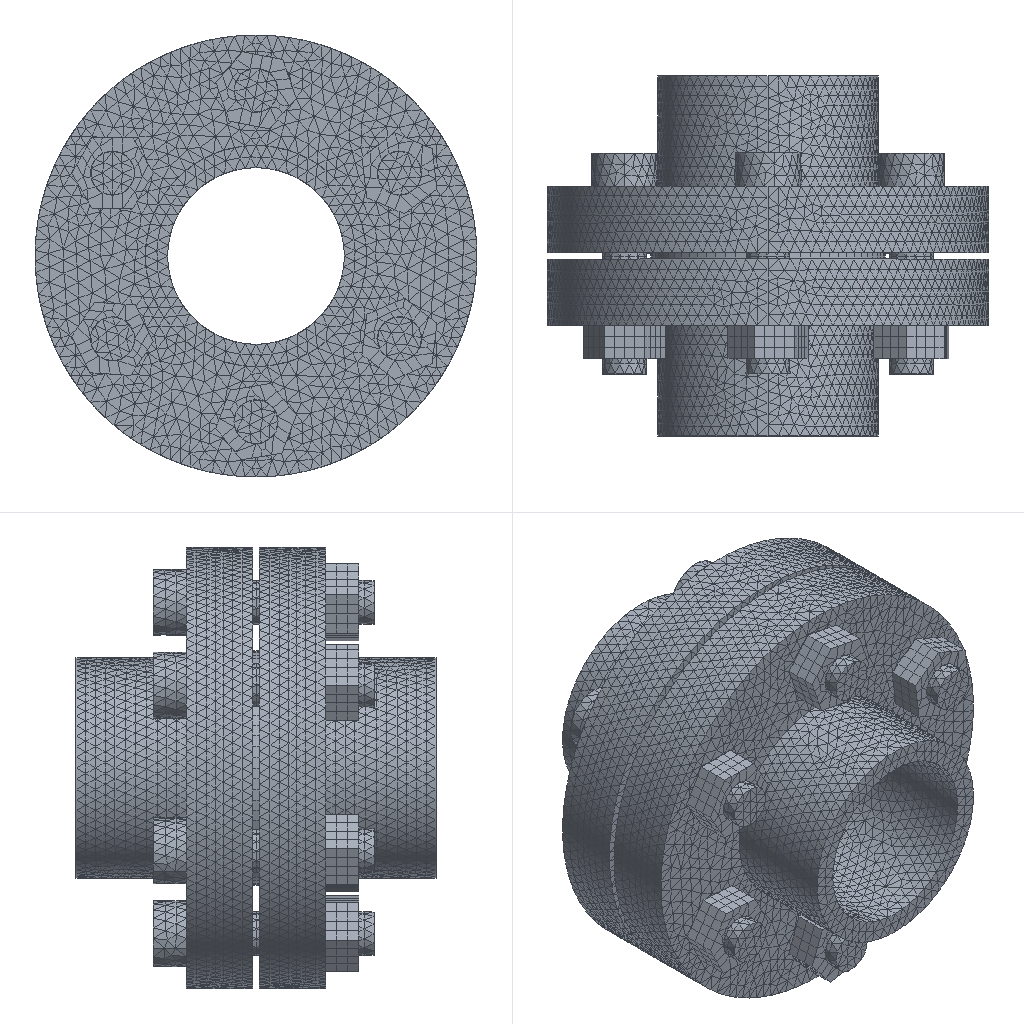Simulation study | ansys workbench
Set-up summary:
category,name,step,type,value,unit,region
solver,ansys_workbench
units,mm-N-s-tonne (MPa),,stated,"/units,MPA"
analysis,LS1,,static
load_step,LS1,LS1,static,nsubst=1; time=1
load_step,LS2,LS2,static,nsubst=1; time=2
mesh,nodes,,,141271
mesh,elements,,,93836
element_type,SOLID187,,,84073
element_type,SURF154,,,4096
element_type,TARGE170,,,2487
element_type,CONTA174,,,2487
element_type,SOLID186,,,693
material,Structural Steel,,E,200000,tonne s^-2 mm^-1
material,Structural Steel,,nu,0.3
material,Structural Steel,,density,7.85e-09,tonne mm^-3
material,Structural Steel,,conductivity,60.5,tonne mm s^-3 C^-1
material,Structural Steel,,specific_heat,4.34e+08,mm^2 s^-2 C^-1
material,Structural Steel,,cte,1.2e-05,C^-1
material,Structural Steel,,permeability,10000
material,Structural Steel,,resistivity,0.00017,ohm mm
material,Y?,,E,43,tonne s^-2 mm^-1
material,Y?,,nu,0.4995
material,Y?,,density,1.2e-09,tonne mm^-3
load,Define Pressure Using Surface Effect Elements,LS1,pressure,0.6,,SURF154 #44
load,Define Force Using Surface Effect Elements,LS1,surface-effect pres face 2,-18.392,,SURF154 #45
load,Define Force Using Surface Effect Elements,LS1,surface-effect pres face 2,-26.88,,SURF154 #46
load,Define Force Using Surface Effect Elements,LS1,surface-effect pres face 2,-26.88,,SURF154 #47
load,Define Force Using Surface Effect Elements,LS1,surface-effect pres face 2,-35.368,,SURF154 #48
load,Define Force Using Surface Effect Elements,LS1,surface-effect pres face 2,-26.88,,SURF154 #49
load,Define Force Using Surface Effect Elements,LS1,surface-effect pres face 2,-26.88,,SURF154 #50
bc,Fixed Supports,model,fixed,[dofs=ALL],,_FIXEDSU
contact,Contact Region,,bonded (always),element=CONTA174
contact,Contact Region 2,,bonded (always),element=CONTA174
contact,Contact Region 3,,bonded (always),element=CONTA174
contact,Contact Region 4,,bonded (always),element=CONTA174
contact,Contact Region 5,,bonded (always),element=CONTA174
contact,Contact Region 6,,bonded (always),element=CONTA174
contact,Contact Region,,bonded (always),element=CONTA174
contact,Contact Region 2,,bonded (always),element=CONTA174
contact,Contact Region 3,,bonded (always),element=CONTA174
contact,Contact Region 4,,bonded (always),element=CONTA174
contact,Contact Region 5,,bonded (always),element=CONTA174
contact,Contact Region 6,,bonded (always),element=CONTA174
contact,Frictional - dianpian ? falan2,,standard (frictionless/frictional),friction=0.15; element=CONTA174
contact,Frictional - dianpian ? falan2,,standard (frictionless/frictional),friction=0.15; element=CONTA174
named_set,_FIXEDSU,,node,3152
gap,solver deck withheld: 4 node/element IDs were masked by the original cleaner and cannot be restored
gap,3 mesh block lines contain redaction underscores in place of numbers (deck corrupted by upstream cleaning)
Ansys APDL input file, long lists of numbers shortened:
/batch
/config,noeldb,1     ! force off writing results to database
*get,_wallstrt,active,,time,wall
! ANSYS input file written by Workbench version 2021 R1
! File used for geometry attach: D:\____\____.__.__________________\______________________\___\_____\__\_____.agdb
/title,________--____ (F5)
! ****** Begin Custom Load Command Snippet ******
/COM, ACT Extensions:
/COM,     LSDYNA, 2021.1
/COM,
! ****** End   Custom Load Command Snippet ******
*DIM,_wb_ProjectScratch_dir,string,248
_wb_ProjectScratch_dir(1) = 'D:\____\____.__.__________________\_______________\_______\_
*DIM,_wb_SolverFiles_dir,string,248
_wb_SolverFiles_dir(1) = 'D:\____\____.__.__________________\______________________\___\_____\____\_
*DIM,_wb_userfiles_dir,string,248
_wb_userfiles_dir(1) = 'D:\____\____.__.__________________\______________________\__________\_
/com,--- Data in consistent NMM units. See Solving Units in the help system for more information.
/units,MPA
/nopr
/wb,file,start              !  signify a WB generated input file
/prep7
! Turn off shape checking because checks already performed inside WB mesher.
! See help system for more information.
SHPP,OFF,,NOWARN
/nolist
etcon,set             ! allow ANSYS to choose best KEYOP's for 180x elements, resets any applicable keyopt to MAPDL defaults
/com,*********** Nodes for the whole assembly ***********
nblock,3,,155398
(1i9,3e20.9e3)
        1    -8.422280547E+00    -4.300000000E+01     8.425544390E+01
! (141270 more lines like these left out)
-1
/wb,elem,start            !  set before creation of elements
/com,*********** Elements for Body 1 "M20-LM" ***********
et,1,186
keyo,1,2,1          ! set full integration on SOLID186
eblock,19,solid,,84
(19i9)
        1        1        1        1        0        0        0        0       20        0      253     1846     1919     1989     1990     1866     1926     1995     1996
! (167 more lines like these left out)
-1
/com,*********** Elements for Body 2 "M20-LM" ***********
et,2,186
keyo,2,2,1          ! set full integration on SOLID186
eblock,19,solid,,81
(19i9)
        2        2        2        2        0        0        0        0       20        0       82      604      676      761      759      624      688      765      764
! (161 more lines like these left out)
-1
/com,*********** Elements for Body 3 "M20-LM" ***********
et,3,186
keyo,3,2,1          ! set full integration on SOLID186
eblock,19,solid,,90
(19i9)
        3        3        3        3        0        0        0        0       20        0     4641     9884     9967    10038    10040     9913     9974    10043    10044
! (179 more lines like these left out)
-1
/com,*********** Elements for Body 4 "M20-LM" ***********
et,4,186
keyo,4,2,1          ! set full integration on SOLID186
eblock,19,solid,,84
(19i9)
        4        4        4        4        0        0        0        0       20        0     4731    10538    10544    10676    10678    10549    10546    10680    10681
! (167 more lines like these left out)
-1
/com,*********** Elements for Body 5 "M20-LM" ***********
et,5,186
keyo,5,2,1          ! set full integration on SOLID186
eblock,19,solid,,81
(19i9)
        5        5        5        5        0        0        0        0       20        0        1        1       73      158      156       21       85      162      161
! (161 more lines like these left out)
-1
/com,*********** Elements for Body 6 "M20-LM" ***********
et,6,186
keyo,6,2,1          ! set full integration on SOLID186
eblock,19,solid,,90
(19i9)
        6        6        6        6        0        0        0        0       20        0      163     1221     1223     1359     1361     1226     1225     1363     1364
! (179 more lines like these left out)
-1
/com,*********** Elements for Body 7 "M20-LD" ***********
et,7,187
eblock,19,solid,,2150
(19i9)
        7        7        7        7        0        0        0        0       10        0     2491     6232     6758     6501     6577     7170     8724     7166     7169
! (4299 more lines like these left out)
-1
/com,*********** Elements for Body 8 "M20-LD" ***********
et,8,187
eblock,19,solid,,2139
(19i9)
        8        8        8        8        0        0        0        0       10        0     4815    11148    11685    11722    11699    11834    14780    11836    11835
! (4277 more lines like these left out)
-1
/com,*********** Elements for Body 9 "M20-LD" ***********
et,9,187
eblock,19,solid,,2154
(19i9)
        9        9        9        9        0        0        0        0       10        0      337     2642     3046     2670     2952     4154     4323     4151     4152
! (4307 more lines like these left out)
-1
/com,*********** Elements for Body 10 "M20-LD" ***********
et,10,187
eblock,19,solid,,2129
(19i9)
       10       10       10       10        0        0        0        0       10        0     6954    15108    15413    15292    15331    17084    18113    17082    17083
! (4257 more lines like these left out)
-1
/com,*********** Elements for Body 11 "M20-LD" ***********
et,11,187
eblock,19,solid,,2131
(19i9)
       11       11       11       11        0        0        0        0       10        0     9083    18647    18648    19090    19085    19937    19949    19944    19943
! (4261 more lines like these left out)
-1
/com,*********** Elements for Body 12 "M20-LD" ***********
et,12,187
eblock,19,solid,,2119
(19i9)
       12       12       12       12        0        0        0        0       10        0    11214    22409    22681    22769    22683    24106    25610    24108    24107
! (4237 more lines like these left out)
-1
/com,*********** Elements for Body 13 "dianpian" ***********
et,13,186
keyo,13,2,1          ! set full integration on SOLID186
eblock,19,solid,,183
(19i9)
       13       13       13       13        0        0        0        0       20        0    13333    25898    25899    25972    25973    26053    26052    25979    25978
! (365 more lines like these left out)
-1
/com,*********** Elements for Body 14 "falan2" ***********
et,14,187
eblock,19,solid,,35806
(19i9)
       14       14       14       14        0        0        0        0       10        0    13516    33716    35796    35004    35246    76246    83049    76243    76244
! (71611 more lines like these left out)
-1
/com,*********** Elements for Body 15 "falan2" ***********
et,15,187
eblock,19,solid,,35445
(19i9)
       15       15       15       15        0        0        0        0       10        0    49322    86725    90133    92904    92212   107151   128857   107153   107152
! (70889 more lines like these left out)
-1
/wb,elem,end               !  done creating elements
/com,*********** Send User Defined Coordinate System(s) ***********
csys,0
toffst,273.15,  ! Temperature offset from absolute zero
/com,*********** Set Reference Temperature ***********
tref,22.
/wb,mat,start              !  starting to send materials
/com,*********** Send Materials ***********
Temperature = 'TEMP' ! Temperature
MP,DENS,1,7.85e-09,	! tonne mm^-3
MP,ALPX,1,1.2e-05,	! C^-1
MP,C,1,434000000,	! mm^2 s^-2 C^-1
MP,KXX,1,60.5,	! tonne mm s^-3 C^-1
MP,RSVX,1,0.00017,	! ohm mm
MP,EX,1,200000,	! tonne s^-2 mm^-1
MP,NUXY,1,0.3,
MP,MURX,1,10000,
Temperature = 'TEMP' ! Temperature
MP,DENS,2,7.85e-09,	! tonne mm^-3
MP,ALPX,2,1.2e-05,	! C^-1
MP,C,2,434000000,	! mm^2 s^-2 C^-1
MP,KXX,2,60.5,	! tonne mm s^-3 C^-1
MP,RSVX,2,0.00017,	! ohm mm
MP,EX,2,200000,	! tonne s^-2 mm^-1
MP,NUXY,2,0.3,
MP,MURX,2,10000,
Temperature = 'TEMP' ! Temperature
MP,DENS,3,7.85e-09,	! tonne mm^-3
MP,ALPX,3,1.2e-05,	! C^-1
MP,C,3,434000000,	! mm^2 s^-2 C^-1
MP,KXX,3,60.5,	! tonne mm s^-3 C^-1
MP,RSVX,3,0.00017,	! ohm mm
MP,EX,3,200000,	! tonne s^-2 mm^-1
MP,NUXY,3,0.3,
MP,MURX,3,10000,
Temperature = 'TEMP' ! Temperature
MP,DENS,4,7.85e-09,	! tonne mm^-3
MP,ALPX,4,1.2e-05,	! C^-1
MP,C,4,434000000,	! mm^2 s^-2 C^-1
MP,KXX,4,60.5,	! tonne mm s^-3 C^-1
MP,RSVX,4,0.00017,	! ohm mm
MP,EX,4,200000,	! tonne s^-2 mm^-1
MP,NUXY,4,0.3,
MP,MURX,4,10000,
Temperature = 'TEMP' ! Temperature
MP,DENS,5,7.85e-09,	! tonne mm^-3
MP,ALPX,5,1.2e-05,	! C^-1
MP,C,5,434000000,	! mm^2 s^-2 C^-1
MP,KXX,5,60.5,	! tonne mm s^-3 C^-1
MP,RSVX,5,0.00017,	! ohm mm
MP,EX,5,200000,	! tonne s^-2 mm^-1
MP,NUXY,5,0.3,
MP,MURX,5,10000,
Temperature = 'TEMP' ! Temperature
MP,DENS,6,7.85e-09,	! tonne mm^-3
MP,ALPX,6,1.2e-05,	! C^-1
MP,C,6,434000000,	! mm^2 s^-2 C^-1
MP,KXX,6,60.5,	! tonne mm s^-3 C^-1
MP,RSVX,6,0.00017,	! ohm mm
MP,EX,6,200000,	! tonne s^-2 mm^-1
MP,NUXY,6,0.3,
MP,MURX,6,10000,
Temperature = 'TEMP' ! Temperature
MP,DENS,7,7.85e-09,	! tonne mm^-3
MP,ALPX,7,1.2e-05,	! C^-1
MP,C,7,434000000,	! mm^2 s^-2 C^-1
MP,KXX,7,60.5,	! tonne mm s^-3 C^-1
MP,RSVX,7,0.00017,	! ohm mm
MP,EX,7,200000,	! tonne s^-2 mm^-1
MP,NUXY,7,0.3,
MP,MURX,7,10000,
Temperature = 'TEMP' ! Temperature
MP,DENS,8,7.85e-09,	! tonne mm^-3
MP,ALPX,8,1.2e-05,	! C^-1
MP,C,8,434000000,	! mm^2 s^-2 C^-1
MP,KXX,8,60.5,	! tonne mm s^-3 C^-1
MP,RSVX,8,0.00017,	! ohm mm
MP,EX,8,200000,	! tonne s^-2 mm^-1
MP,NUXY,8,0.3,
MP,MURX,8,10000,
Temperature = 'TEMP' ! Temperature
MP,DENS,9,7.85e-09,	! tonne mm^-3
MP,ALPX,9,1.2e-05,	! C^-1
MP,C,9,434000000,	! mm^2 s^-2 C^-1
MP,KXX,9,60.5,	! tonne mm s^-3 C^-1
MP,RSVX,9,0.00017,	! ohm mm
MP,EX,9,200000,	! tonne s^-2 mm^-1
MP,NUXY,9,0.3,
MP,MURX,9,10000,
Temperature = 'TEMP' ! Temperature
MP,DENS,10,7.85e-09,	! tonne mm^-3
MP,ALPX,10,1.2e-05,	! C^-1
MP,C,10,434000000,	! mm^2 s^-2 C^-1
MP,KXX,10,60.5,	! tonne mm s^-3 C^-1
MP,RSVX,10,0.00017,	! ohm mm
MP,EX,10,200000,	! tonne s^-2 mm^-1
MP,NUXY,10,0.3,
MP,MURX,10,10000,
Temperature = 'TEMP' ! Temperature
MP,DENS,11,7.85e-09,	! tonne mm^-3
MP,ALPX,11,1.2e-05,	! C^-1
MP,C,11,434000000,	! mm^2 s^-2 C^-1
MP,KXX,11,60.5,	! tonne mm s^-3 C^-1
MP,RSVX,11,0.00017,	! ohm mm
MP,EX,11,200000,	! tonne s^-2 mm^-1
MP,NUXY,11,0.3,
MP,MURX,11,10000,
Temperature = 'TEMP' ! Temperature
MP,DENS,12,7.85e-09,	! tonne mm^-3
MP,ALPX,12,1.2e-05,	! C^-1
MP,C,12,434000000,	! mm^2 s^-2 C^-1
MP,KXX,12,60.5,	! tonne mm s^-3 C^-1
MP,RSVX,12,0.00017,	! ohm mm
MP,EX,12,200000,	! tonne s^-2 mm^-1
MP,NUXY,12,0.3,
MP,MURX,12,10000,
MP,DENS,13,1.2e-09,	! tonne mm^-3
MP,EX,13,43,	! tonne s^-2 mm^-1
MP,NUXY,13,0.4995,
Temperature = 'TEMP' ! Temperature
MP,DENS,14,7.85e-09,	! tonne mm^-3
MP,ALPX,14,1.2e-05,	! C^-1
MP,C,14,434000000,	! mm^2 s^-2 C^-1
MP,KXX,14,60.5,	! tonne mm s^-3 C^-1
MP,RSVX,14,0.00017,	! ohm mm
MP,EX,14,200000,	! tonne s^-2 mm^-1
MP,NUXY,14,0.3,
MP,MURX,14,10000,
Temperature = 'TEMP' ! Temperature
MP,DENS,15,7.85e-09,	! tonne mm^-3
MP,ALPX,15,1.2e-05,	! C^-1
MP,C,15,434000000,	! mm^2 s^-2 C^-1
MP,KXX,15,60.5,	! tonne mm s^-3 C^-1
MP,RSVX,15,0.00017,	! ohm mm
MP,EX,15,200000,	! tonne s^-2 mm^-1
MP,NUXY,15,0.3,
MP,MURX,15,10000,
/wb,mat,end                !  done sending materials
!************************* Model Summary ********************
!M20-LM,	结构钢,	matid,	1
!M20-LM,	结构钢,	matid,	2
!M20-LM,	结构钢,	matid,	3
!M20-LM,	结构钢,	matid,	4
!M20-LM,	结构钢,	matid,	5
!M20-LM,	结构钢,	matid,	6
!M20-LD,	结构钢,	matid,	7
!M20-LD,	结构钢,	matid,	8
!M20-LD,	结构钢,	matid,	9
!M20-LD,	结构钢,	matid,	10
!M20-LD,	结构钢,	matid,	11
!M20-LD,	结构钢,	matid,	12
!dianpian,	Y形圈,	matid,	13
!falan2,	结构钢,	matid,	14
!falan2,	结构钢,	matid,	15
!************************* End Model Summary ********************
! get the diagonal of the bounding box. Needed later for other things
*get,_xmin,node,,mnloc,x
*get,_ymin,node,,mnloc,y
*get,_zmin,node,,mnloc,z
*get,_xmax,node,,mxloc,x
*get,_ymax,node,,mxloc,y
*get,_zmax,node,,mxloc,z
_ASMDIAG=(_xmax-_xmin)*(_xmax-_xmin)+(_ymax-_ymin)*(_ymax-_ymin)+(_zmax-_zmin)*(_zmax-_zmin)
_ASMDIAG=SQRT(_ASMDIAG)
/wb,contact,start          !  starting to send contact
/com,*********** Create Contact "接触区域" ***********
/com,            Real Constant Set For Above Contact Is 17 & 16
*set,tid,17
*set,cid,16
r,tid
r,cid
et,tid,170
et,cid,174
eblock,10,,,34
(15i9)
   109337       17       17       17        0     6176     6221     6177     6177     6795     6809     6177     6794
! (33 more lines like these left out)
-1
eblock,10,,,34
(15i9)
   109371       16       16       16        0     6176     6221     6177     6177     6795     6809     6177     6794
! (33 more lines like these left out)
-1
eblock,10,,,55
(15i9)
   109405       16       17       16        0    88589    88847    88848    88848   119179   121126    88848   119180
! (54 more lines like these left out)
-1
eblock,10,,,55
(15i9)
   109460       17       16       17        0    88589    88847    88848    88848   119179   121126    88848   119180
! (54 more lines like these left out)
-1
keyo,cid,8,2               ! auto create asymmetric contact (from Program Controlled setting)
keyo,cid,10,0              ! adjust contact stiffness each NR iteration (from Program Controlled setting)
keyo,cid,12,5              ! bonded always
keyo,cid,18,1              ! small sliding turned on by application
keyo,cid,2,0               ! augmented Lagrange (from Program Controlled setting)
keyo,cid,4,0               ! on Gauss point (from Program Controlled setting)
keyo,cid,9,1               ! ignore initial gaps/penetration
keyo,cid,7,0               ! No Prediction
rmod,tid,3,1.       ! FKN
rmod,tid,5,0.       ! ICONT
rmod,tid,6,0.       ! PINB
rmod,tid,10,0.      ! CNOF
rmod,tid,12,0.      ! FKT
rmod,tid,36,1539    ! WB DSID
rmod,cid,3,1.       ! FKN
rmod,cid,5,0.       ! ICONT
rmod,cid,6,0.       ! PINB
rmod,cid,10,0.      ! CNOF
rmod,cid,12,0.      ! FKT
rmod,cid,36,1539    ! WB DSID
/com,*********** Create Contact "接触区域 2" ***********
/com,            Real Constant Set For Above Contact Is 19 & 18
*set,tid,19
*set,cid,18
r,tid
r,cid
et,tid,170
et,cid,174
eblock,10,,,34
(15i9)
   109515       19       19       19        0    11142    11187    11143    11143    11758    11772    11143    11757
! (33 more lines like these left out)
-1
eblock,10,,,34
(15i9)
   109549       18       18       18        0    11142    11187    11143    11143    11758    11772    11143    11757
! (33 more lines like these left out)
-1
eblock,10,,,50
(15i9)
   109583       18       19       18        0    88701    88827    89030    89030   120181   121009    89030   120184
! (49 more lines like these left out)
-1
eblock,10,,,50
(15i9)
   109633       19       18       19        0    88701    88827    89030    89030   120181   121009    89030   120184
! (49 more lines like these left out)
-1
keyo,cid,8,2               ! auto create asymmetric contact (from Program Controlled setting)
keyo,cid,10,0              ! adjust contact stiffness each NR iteration (from Program Controlled setting)
keyo,cid,12,5              ! bonded always
keyo,cid,18,1              ! small sliding turned on by application
keyo,cid,2,0               ! augmented Lagrange (from Program Controlled setting)
keyo,cid,4,0               ! on Gauss point (from Program Controlled setting)
keyo,cid,9,1               ! ignore initial gaps/penetration
keyo,cid,7,0               ! No Prediction
rmod,tid,3,1.       ! FKN
rmod,tid,5,0.       ! ICONT
rmod,tid,6,0.       ! PINB
rmod,tid,10,0.      ! CNOF
rmod,tid,12,0.      ! FKT
rmod,tid,36,1542    ! WB DSID
rmod,cid,3,1.       ! FKN
rmod,cid,5,0.       ! ICONT
rmod,cid,6,0.       ! PINB
rmod,cid,10,0.      ! CNOF
rmod,cid,12,0.      ! FKT
rmod,cid,36,1542    ! WB DSID
/com,*********** Create Contact "接触区域 3" ***********
/com,            Real Constant Set For Above Contact Is 21 & 20
*set,tid,21
*set,cid,20
r,tid
r,cid
et,tid,170
et,cid,174
eblock,10,,,34
(15i9)
   109683       21       21       21        0     2465     2510     2466     2466     3083     3096     2466     3082
! (33 more lines like these left out)
-1
eblock,10,,,34
(15i9)
   109717       20       20       20        0     2465     2510     2466     2466     3083     3096     2466     3082
! (33 more lines like these left out)
-1
eblock,10,,,51
(15i9)
   109751       20       21       20        0    88735    89087    89049    89049   120431   122030    89049   120429
! (50 more lines like these left out)
-1
eblock,10,,,51
(15i9)
   109802       21       20       21        0    88735    89087    89049    89049   120431   122030    89049   120429
! (50 more lines like these left out)
-1
keyo,cid,8,2               ! auto create asymmetric contact (from Program Controlled setting)
keyo,cid,10,0              ! adjust contact stiffness each NR iteration (from Program Controlled setting)
keyo,cid,12,5              ! bonded always
keyo,cid,18,1              ! small sliding turned on by application
keyo,cid,2,0               ! augmented Lagrange (from Program Controlled setting)
keyo,cid,4,0               ! on Gauss point (from Program Controlled setting)
keyo,cid,9,1               ! ignore initial gaps/penetration
keyo,cid,7,0               ! No Prediction
rmod,tid,3,1.       ! FKN
rmod,tid,5,0.       ! ICONT
rmod,tid,6,0.       ! PINB
rmod,tid,10,0.      ! CNOF
rmod,tid,12,0.      ! FKT
rmod,tid,36,1545    ! WB DSID
rmod,cid,3,1.       ! FKN
rmod,cid,5,0.       ! ICONT
rmod,cid,6,0.       ! PINB
rmod,cid,10,0.      ! CNOF
rmod,cid,12,0.      ! FKT
rmod,cid,36,1545    ! WB DSID
/com,*********** Create Contact "接触区域 4" ***********
/com,            Real Constant Set For Above Contact Is 23 & 22
*set,tid,23
*set,cid,22
r,tid
r,cid
et,tid,170
et,cid,174
eblock,10,,,34
(15i9)
   109853       23       23       23        0    14836    14881    14837    14837    15449    15461    14837    15448
! (33 more lines like these left out)
-1
eblock,10,,,34
(15i9)
   109887       22       22       22        0    14836    14881    14837    14837    15449    15461    14837    15448
! (33 more lines like these left out)
-1
eblock,10,,,51
(15i9)
   109921       22       23       22        0    88641    88829    89093    89093   119655   121022    89093   119657
! (50 more lines like these left out)
-1
eblock,10,,,51
(15i9)
   109972       23       22       23        0    88641    88829    89093    89093   119655   121022    89093   119657
! (50 more lines like these left out)
-1
keyo,cid,8,2               ! auto create asymmetric contact (from Program Controlled setting)
keyo,cid,10,0              ! adjust contact stiffness each NR iteration (from Program Controlled setting)
keyo,cid,12,5              ! bonded always
keyo,cid,18,1              ! small sliding turned on by application
keyo,cid,2,0               ! augmented Lagrange (from Program Controlled setting)
keyo,cid,4,0               ! on Gauss point (from Program Controlled setting)
keyo,cid,9,1               ! ignore initial gaps/penetration
keyo,cid,7,0               ! No Prediction
rmod,tid,3,1.       ! FKN
rmod,tid,5,0.       ! ICONT
rmod,tid,6,0.       ! PINB
rmod,tid,10,0.      ! CNOF
rmod,tid,12,0.      ! FKT
rmod,tid,36,1548    ! WB DSID
rmod,cid,3,1.       ! FKN
rmod,cid,5,0.       ! ICONT
rmod,cid,6,0.       ! PINB
rmod,cid,10,0.      ! CNOF
rmod,cid,12,0.      ! FKT
rmod,cid,36,1548    ! WB DSID
/com,*********** Create Contact "接触区域 5" ***********
/com,            Real Constant Set For Above Contact Is 25 & 24
*set,tid,25
*set,cid,24
r,tid
r,cid
et,tid,170
et,cid,174
eblock,10,,,34
(15i9)
   110023       25       25       25        0    18513    18558    18514    18514    19128    19140    18514    19127
! (33 more lines like these left out)
-1
eblock,10,,,34
(15i9)
   110057       24       24       24        0    18513    18558    18514    18514    19128    19140    18514    19127
! (33 more lines like these left out)
-1
eblock,10,,,55
(15i9)
   110091       24       25       24        0    88730    88964    88965    88965   120392   121699    88965   120393
! (54 more lines like these left out)
-1
eblock,10,,,55
(15i9)
   110146       25       24       25        0    88730    88964    88965    88965   120392   121699    88965   120393
! (54 more lines like these left out)
-1
keyo,cid,8,2               ! auto create asymmetric contact (from Program Controlled setting)
keyo,cid,10,0              ! adjust contact stiffness each NR iteration (from Program Controlled setting)
keyo,cid,12,5              ! bonded always
keyo,cid,18,1              ! small sliding turned on by application
keyo,cid,2,0               ! augmented Lagrange (from Program Controlled setting)
keyo,cid,4,0               ! on Gauss point (from Program Controlled setting)
keyo,cid,9,1               ! ignore initial gaps/penetration
keyo,cid,7,0               ! No Prediction
rmod,tid,3,1.       ! FKN
rmod,tid,5,0.       ! ICONT
rmod,tid,6,0.       ! PINB
rmod,tid,10,0.      ! CNOF
rmod,tid,12,0.      ! FKT
rmod,tid,36,1551    ! WB DSID
rmod,cid,3,1.       ! FKN
rmod,cid,5,0.       ! ICONT
rmod,cid,6,0.       ! PINB
rmod,cid,10,0.      ! CNOF
rmod,cid,12,0.      ! FKT
rmod,cid,36,1551    ! WB DSID
/com,*********** Create Contact "接触区域 6" ***********
/com,            Real Constant Set For Above Contact Is 27 & 26
*set,tid,27
*set,cid,26
r,tid
r,cid
et,tid,170
et,cid,174
eblock,10,,,34
(15i9)
   110201       27       27       27        0    22193    22238    22194    22194    22805    22816    22194    22804
! (33 more lines like these left out)
-1
eblock,10,,,34
(15i9)
   110235       26       26       26        0    22193    22238    22194    22194    22805    22816    22194    22804
! (33 more lines like these left out)
-1
eblock,10,,,49
(15i9)
   110269       26       27       26        0    84741    88702    84742    84742    94051    94058    84742    94048
! (48 more lines like these left out)
-1
eblock,10,,,49
(15i9)
   110318       27       26       27        0    84741    88702    84742    84742    94051    94058    84742    94048
! (48 more lines like these left out)
-1
keyo,cid,8,2               ! auto create asymmetric contact (from Program Controlled setting)
keyo,cid,10,0              ! adjust contact stiffness each NR iteration (from Program Controlled setting)
keyo,cid,12,5              ! bonded always
keyo,cid,18,1              ! small sliding turned on by application
keyo,cid,2,0               ! augmented Lagrange (from Program Controlled setting)
keyo,cid,4,0               ! on Gauss point (from Program Controlled setting)
keyo,cid,9,1               ! ignore initial gaps/penetration
keyo,cid,7,0               ! No Prediction
rmod,tid,3,1.       ! FKN
rmod,tid,5,0.       ! ICONT
rmod,tid,6,0.       ! PINB
rmod,tid,10,0.      ! CNOF
rmod,tid,12,0.      ! FKT
rmod,tid,36,1554    ! WB DSID
rmod,cid,3,1.       ! FKN
rmod,cid,5,0.       ! ICONT
rmod,cid,6,0.       ! PINB
rmod,cid,10,0.      ! CNOF
rmod,cid,12,0.      ! FKT
rmod,cid,36,1554    ! WB DSID
/com,*********** Create Contact "接触区域" ***********
/com,            Real Constant Set For Above Contact Is 29 & 28
*set,tid,29
*set,cid,28
r,tid
r,cid
et,tid,170
et,cid,174
eblock,10,,,42
(15i9)
   110367       29       29       29        0     1934     1914     1932     1933     2236     2235     2281     2284
! (41 more lines like these left out)
-1
eblock,10,,,42
(15i9)
   110409       28       28       28        0     1934     1914     1932     1933     2236     2235     2281     2284
! (41 more lines like these left out)
-1
eblock,10,,,112
(15i9)
   110451       28       29       28        0    11218    11212    11241    11241    12195    12197    11241    12235
! (111 more lines like these left out)
-1
eblock,10,,,112
(15i9)
   110563       29       28       29        0    11218    11212    11241    11241    12195    12197    11241    12235
! (111 more lines like these left out)
-1
keyo,cid,8,2               ! auto create asymmetric contact (from Program Controlled setting)
keyo,cid,10,0              ! adjust contact stiffness each NR iteration (from Program Controlled setting)
keyo,cid,12,5              ! bonded always
keyo,cid,18,1              ! small sliding turned on by application
keyo,cid,2,0               ! augmented Lagrange (from Program Controlled setting)
keyo,cid,4,0               ! on Gauss point (from Program Controlled setting)
keyo,cid,9,1               ! ignore initial gaps/penetration
keyo,cid,7,0               ! No Prediction
rmod,tid,3,1.       ! FKN
rmod,tid,5,0.       ! ICONT
rmod,tid,6,0.       ! PINB
rmod,tid,10,0.      ! CNOF
rmod,tid,12,0.      ! FKT
rmod,tid,36,1559    ! WB DSID
rmod,cid,3,1.       ! FKN
rmod,cid,5,0.       ! ICONT
rmod,cid,6,0.       ! PINB
rmod,cid,10,0.      ! CNOF
rmod,cid,12,0.      ! FKT
rmod,cid,36,1559    ! WB DSID
/com,*********** Create Contact "接触区域 2" ***********
/com,            Real Constant Set For Above Contact Is 31 & 30
*set,tid,31
*set,cid,30
r,tid
r,cid
et,tid,170
et,cid,174
eblock,10,,,42
(15i9)
   110675       31       31       31        0      690      670      669      668      974      971      969      970
! (41 more lines like these left out)
-1
eblock,10,,,42
(15i9)
   110717       30       30       30        0      690      670      669      668      974      971      969      970
! (41 more lines like these left out)
-1
eblock,10,,,112
(15i9)
   110759       30       31       30        0     6261     6245     6273     6273     7225     7226     6273     7330
! (111 more lines like these left out)
-1
eblock,10,,,112
(15i9)
   110871       31       30       31        0     6261     6245     6273     6273     7225     7226     6273     7330
! (111 more lines like these left out)
-1
keyo,cid,8,2               ! auto create asymmetric contact (from Program Controlled setting)
keyo,cid,10,0              ! adjust contact stiffness each NR iteration (from Program Controlled setting)
keyo,cid,12,5              ! bonded always
keyo,cid,18,1              ! small sliding turned on by application
keyo,cid,2,0               ! augmented Lagrange (from Program Controlled setting)
keyo,cid,4,0               ! on Gauss point (from Program Controlled setting)
keyo,cid,9,1               ! ignore initial gaps/penetration
keyo,cid,7,0               ! No Prediction
rmod,tid,3,1.       ! FKN
rmod,tid,5,0.       ! ICONT
rmod,tid,6,0.       ! PINB
rmod,tid,10,0.      ! CNOF
rmod,tid,12,0.      ! FKT
rmod,tid,36,1562    ! WB DSID
rmod,cid,3,1.       ! FKN
rmod,cid,5,0.       ! ICONT
rmod,cid,6,0.       ! PINB
rmod,cid,10,0.      ! CNOF
rmod,cid,12,0.      ! FKT
rmod,cid,36,1562    ! WB DSID
/com,*********** Create Contact "接触区域 3" ***********
/com,            Real Constant Set For Above Contact Is 33 & 32
*set,tid,33
*set,cid,32
r,tid
r,cid
et,tid,170
et,cid,174
eblock,10,,,42
(15i9)
   110983       33       33       33        0     9982     9962     9980     9981    10309    10308    10347    10348
! (41 more lines like these left out)
-1
eblock,10,,,42
(15i9)
   111025       32       32       32        0     9982     9962     9980     9981    10309    10308    10347    10348
! (41 more lines like these left out)
-1
eblock,10,,,112
(15i9)
   111067       32       33       32        0     2541     2535     2564     2564     3512     3514     2564     3550
! (111 more lines like these left out)
-1
eblock,10,,,112
(15i9)
   111179       33       32       33        0     2541     2535     2564     2564     3512     3514     2564     3550
! (111 more lines like these left out)
-1
keyo,cid,8,2               ! auto create asymmetric contact (from Program Controlled setting)
keyo,cid,10,0              ! adjust contact stiffness each NR iteration (from Program Controlled setting)
keyo,cid,12,5              ! bonded always
keyo,cid,18,1              ! small sliding turned on by application
keyo,cid,2,0               ! augmented Lagrange (from Program Controlled setting)
keyo,cid,4,0               ! on Gauss point (from Program Controlled setting)
keyo,cid,9,1               ! ignore initial gaps/penetration
keyo,cid,7,0               ! No Prediction
rmod,tid,3,1.       ! FKN
rmod,tid,5,0.       ! ICONT
rmod,tid,6,0.       ! PINB
rmod,tid,10,0.      ! CNOF
rmod,tid,12,0.      ! FKT
rmod,tid,36,1565    ! WB DSID
rmod,cid,3,1.       ! FKN
rmod,cid,5,0.       ! ICONT
rmod,cid,6,0.       ! PINB
rmod,cid,10,0.      ! CNOF
rmod,cid,12,0.      ! FKT
rmod,cid,36,1565    ! WB DSID
/com,*********** Create Contact "接触区域 4" ***********
/com,            Real Constant Set For Above Contact Is 35 & 34
*set,tid,35
*set,cid,34
r,tid
r,cid
et,tid,170
et,cid,174
eblock,10,,,42
(15i9)
   111291       35       35       35        0    10618    10598    10616    10617    10916    10915    10954    10955
! (41 more lines like these left out)
-1
eblock,10,,,42
(15i9)
   111333       34       34       34        0    10618    10598    10616    10617    10916    10915    10954    10955
! (41 more lines like these left out)
-1
eblock,10,,,112
(15i9)
   111375       34       35       34        0    14923    14906    14935    14935    15879    15880    14935    15980
! (111 more lines like these left out)
-1
eblock,10,,,112
(15i9)
   111487       35       34       35        0    14923    14906    14935    14935    15879    15880    14935    15980
! (111 more lines like these left out)
-1
keyo,cid,8,2               ! auto create asymmetric contact (from Program Controlled setting)
keyo,cid,10,0              ! adjust contact stiffness each NR iteration (from Program Controlled setting)
keyo,cid,12,5              ! bonded always
keyo,cid,18,1              ! small sliding turned on by application
keyo,cid,2,0               ! augmented Lagrange (from Program Controlled setting)
keyo,cid,4,0               ! on Gauss point (from Program Controlled setting)
keyo,cid,9,1               ! ignore initial gaps/penetration
keyo,cid,7,0               ! No Prediction
rmod,tid,3,1.       ! FKN
rmod,tid,5,0.       ! ICONT
rmod,tid,6,0.       ! PINB
rmod,tid,10,0.      ! CNOF
rmod,tid,12,0.      ! FKT
rmod,tid,36,1568    ! WB DSID
rmod,cid,3,1.       ! FKN
rmod,cid,5,0.       ! ICONT
rmod,cid,6,0.       ! PINB
rmod,cid,10,0.      ! CNOF
rmod,cid,12,0.      ! FKT
rmod,cid,36,1568    ! WB DSID
/com,*********** Create Contact "接触区域 5" ***********
/com,            Real Constant Set For Above Contact Is 37 & 36
*set,tid,37
*set,cid,36
r,tid
r,cid
et,tid,170
et,cid,174
eblock,10,,,42
(15i9)
   111599       37       37       37        0       87       67       66       65      371      368      366      367
! (41 more lines like these left out)
-1
eblock,10,,,42
(15i9)
   111641       36       36       36        0       87       67       66       65      371      368      366      367
! (41 more lines like these left out)
-1
eblock,10,,,112
(15i9)
   111683       36       37       36        0    18589    18582    18610    18610    19552    19554    18610    19596
! (111 more lines like these left out)
-1
eblock,10,,,112
(15i9)
   111795       37       36       37        0    18589    18582    18610    18610    19552    19554    18610    19596
! (111 more lines like these left out)
-1
keyo,cid,8,2               ! auto create asymmetric contact (from Program Controlled setting)
keyo,cid,10,0              ! adjust contact stiffness each NR iteration (from Program Controlled setting)
keyo,cid,12,5              ! bonded always
keyo,cid,18,1              ! small sliding turned on by application
keyo,cid,2,0               ! augmented Lagrange (from Program Controlled setting)
keyo,cid,4,0               ! on Gauss point (from Program Controlled setting)
keyo,cid,9,1               ! ignore initial gaps/penetration
keyo,cid,7,0               ! No Prediction
rmod,tid,3,1.       ! FKN
rmod,tid,5,0.       ! ICONT
rmod,tid,6,0.       ! PINB
rmod,tid,10,0.      ! CNOF
rmod,tid,12,0.      ! FKT
rmod,tid,36,1571    ! WB DSID
rmod,cid,3,1.       ! FKN
rmod,cid,5,0.       ! ICONT
rmod,cid,6,0.       ! PINB
rmod,cid,10,0.      ! CNOF
rmod,cid,12,0.      ! FKT
rmod,cid,36,1571    ! WB DSID
/com,*********** Create Contact "接触区域 6" ***********
/com,            Real Constant Set For Above Contact Is 39 & 38
*set,tid,39
*set,cid,38
r,tid
r,cid
et,tid,170
et,cid,174
eblock,10,,,42
(15i9)
   111907       39       39       39        0     1301     1281     1299     1300     1636     1635     1674     1675
! (41 more lines like these left out)
-1
eblock,10,,,42
(15i9)
   111949       38       38       38        0     1301     1281     1299     1300     1636     1635     1674     1675
! (41 more lines like these left out)
-1
eblock,10,,,112
(15i9)
   111991       38       39       38        0    22283    22263    22292    22292    23237    23238    22292    23359
! (111 more lines like these left out)
-1
eblock,10,,,112
(15i9)
   112103       39       38       39        0    22283    22263    22292    22292    23237    23238    22292    23359
! (111 more lines like these left out)
-1
keyo,cid,8,2               ! auto create asymmetric contact (from Program Controlled setting)
keyo,cid,10,0              ! adjust contact stiffness each NR iteration (from Program Controlled setting)
keyo,cid,12,5              ! bonded always
keyo,cid,18,1              ! small sliding turned on by application
keyo,cid,2,0               ! augmented Lagrange (from Program Controlled setting)
keyo,cid,4,0               ! on Gauss point (from Program Controlled setting)
keyo,cid,9,1               ! ignore initial gaps/penetration
keyo,cid,7,0               ! No Prediction
rmod,tid,3,1.       ! FKN
rmod,tid,5,0.       ! ICONT
rmod,tid,6,0.       ! PINB
rmod,tid,10,0.      ! CNOF
rmod,tid,12,0.      ! FKT
rmod,tid,36,1574    ! WB DSID
rmod,cid,3,1.       ! FKN
rmod,cid,5,0.       ! ICONT
rmod,cid,6,0.       ! PINB
rmod,cid,10,0.      ! CNOF
rmod,cid,12,0.      ! FKT
rmod,cid,36,1574    ! WB DSID
/com,*********** Create Contact "摩擦的 - dianpian 至 falan2" ***********
/com,            Real Constant Set For Above Contact Is 41 & 40
*set,tid,41
*set,cid,40
r,tid
r,cid
et,tid,170
et,cid,174
eblock,10,,,183
(15i9)
   112215       41       41       41        0    25908    25965    25909    25909    26542    26546    25909    26541
! (182 more lines like these left out)
-1
eblock,10,,,183
(15i9)
   112398       40       40       40        0    25908    25965    25909    25909    26542    26546    25909    26541
! (182 more lines like these left out)
-1
eblock,10,,,341
(15i9)
   112581       40       41       40        0    30790    30876    31010    31010    58112    58879    31010    58114
! (340 more lines like these left out)
-1
eblock,10,,,341
(15i9)
   112922       41       40       41        0    30790    30876    31010    31010    58112    58879    31010    58114
! (340 more lines like these left out)
-1
keyo,cid,8,2               ! auto create asymmetric contact (from Program Controlled setting)
keyo,cid,10,0              ! adjust contact stiffness each NR iteration (from Program Controlled setting)
keyo,cid,12,0              ! standard contact
mp,mu,cid,0.15      ! unitless
keyo,cid,18,1              ! small sliding turned on by application
keyo,cid,2,0               ! augmented Lagrange (from Program Controlled setting)
keyo,cid,4,0               ! on Gauss point (from Program Controlled setting)
keyo,cid,9,0               ! use real geometry with stepped effects
keyo,cid,7,0               ! No Prediction
rmod,tid,3,1.       ! FKN
rmod,tid,5,0.       ! ICONT
rmod,tid,6,0.       ! PINB
rmod,tid,10,0.      ! CNOF
rmod,tid,12,0.      ! FKT
rmod,tid,36,1579    ! WB DSID
rmod,cid,3,1.       ! FKN
rmod,cid,5,0.       ! ICONT
rmod,cid,6,0.       ! PINB
rmod,cid,10,0.      ! CNOF
rmod,cid,12,0.      ! FKT
rmod,cid,36,1579    ! WB DSID
/com,*********** Create Contact "摩擦的 - dianpian 至 falan2" ***********
/com,            Real Constant Set For Above Contact Is 43 & 42
*set,tid,43
*set,cid,42
r,tid
r,cid
et,tid,170
et,cid,174
eblock,10,,,183
(15i9)
   113263       43       43       43        0    26043    26042    25986    25986    26955    26793    25986    26794
! (182 more lines like these left out)
-1
eblock,10,,,183
(15i9)
   113446       42       42       42        0    26043    26042    25986    25986    26955    26793    25986    26794
! (182 more lines like these left out)
-1
eblock,10,,,341
(15i9)
   113629       42       43       42        0    87950    88036    88170    88170   115112   115873    88170   115114
! (340 more lines like these left out)
-1
eblock,10,,,341
(15i9)
   113970       43       42       43        0    87950    88036    88170    88170   115112   115873    88170   115114
! (340 more lines like these left out)
-1
keyo,cid,8,2               ! auto create asymmetric contact (from Program Controlled setting)
keyo,cid,10,0              ! adjust contact stiffness each NR iteration (from Program Controlled setting)
keyo,cid,12,0              ! standard contact
mp,mu,cid,0.15      ! unitless
keyo,cid,18,1              ! small sliding turned on by application
keyo,cid,2,0               ! augmented Lagrange (from Program Controlled setting)
keyo,cid,4,0               ! on Gauss point (from Program Controlled setting)
keyo,cid,9,0               ! use real geometry with stepped effects
keyo,cid,7,0               ! No Prediction
rmod,tid,3,1.       ! FKN
rmod,tid,5,0.       ! ICONT
rmod,tid,6,0.       ! PINB
rmod,tid,10,0.      ! CNOF
rmod,tid,12,0.      ! FKT
rmod,tid,36,1582    ! WB DSID
rmod,cid,3,1.       ! FKN
rmod,cid,5,0.       ! ICONT
rmod,cid,6,0.       ! PINB
rmod,cid,10,0.      ! CNOF
rmod,cid,12,0.      ! FKT
rmod,cid,36,1582    ! WB DSID
nsel,all
esel,all
/wb,contact,end            !  done creating contacts
/golist
/wb,load,start             !  starting to send loads
/com,*********** Fixed Supports ***********
CMBLOCK,_FIXEDSU,NODE,     3152
(8i10)
     27514     27520     27521     27522     27523     27524     27525     27526
! (393 more lines like these left out)
cmsel,s,_FIXEDSU
d,all,all
nsel,all
/com,*********** Define Pressure Using Surface Effect Elements ***********
et,44,154
eblock,10,,,3700
(15i9)
   114311       44       44       44        0    84592    84591    87504    87504    92931    92933    87504    92937
! (3699 more lines like these left out)
-1
esel,s,type,,44
keyop,44,7,0                ! Use deformed area for application of load
esel,all
*DIM,_loadvari835,TABLE,3,1,1,TIME,
! Time values
_loadvari835(1,0,1) = 0.
_loadvari835(2,0,1) = 1.
_loadvari835(3,0,1) = 2.
! Load values
_loadvari835(1,1,1) = 0.
_loadvari835(2,1,1) = 0.
_loadvari835(3,1,1) = 0.6
/com,*********** Define Force Using Surface Effect Elements ***********
local,12,0,0.,0.,0.,0.,0.,0.
csys,0
et,45,154
eblock,10,,,66
(15i9)
   118011       45       45       45       12    11505    11528    11515    11515    13870    13945    11515    13868
! (65 more lines like these left out)
-1
esel,s,type,,45
keyop,45,2,1                ! Apply load in local coordinate system
keyop,45,7,1                ! Use original area so load is constant in large deformation
esel,all
*DIM,_loadvari871x,TABLE,3,1,1,TIME,
! Time values
_loadvari871x(1,0,1) = 0.
_loadvari871x(2,0,1) = 1.
_loadvari871x(3,0,1) = 2.
! Load values
_loadvari871x(1,1,1) = 0.
_loadvari871x(2,1,1) = 0.
_loadvari871x(3,1,1) = 0.
*DIM,_loadvari871y,TABLE,3,1,1,TIME,
! Time values
_loadvari871y(1,0,1) = 0.
_loadvari871y(2,0,1) = 1.
_loadvari871y(3,0,1) = 2.
! Load values
_loadvari871y(1,1,1) = 0.
_loadvari871y(2,1,1) = -18.392
_loadvari871y(3,1,1) = -18.392
*DIM,_loadvari871z,TABLE,3,1,1,TIME,
! Time values
_loadvari871z(1,0,1) = 0.
_loadvari871z(2,0,1) = 1.
_loadvari871z(3,0,1) = 2.
! Load values
_loadvari871z(1,1,1) = 0.
_loadvari871z(2,1,1) = 0.
_loadvari871z(3,1,1) = 0.
/com,*********** Define Force Using Surface Effect Elements ***********
local,13,0,0.,0.,0.,0.,0.,0.
csys,0
et,46,154
eblock,10,,,66
(15i9)
   118077       46       46       46       13     6541     6564     6551     6551     8915     8983     6551     8913
! (65 more lines like these left out)
-1
esel,s,type,,46
keyop,46,2,1                ! Apply load in local coordinate system
keyop,46,7,1                ! Use original area so load is constant in large deformation
esel,all
*DIM,_loadvari879x,TABLE,3,1,1,TIME,
! Time values
_loadvari879x(1,0,1) = 0.
_loadvari879x(2,0,1) = 1.
_loadvari879x(3,0,1) = 2.
! Load values
_loadvari879x(1,1,1) = 0.
_loadvari879x(2,1,1) = 0.
_loadvari879x(3,1,1) = 0.
*DIM,_loadvari879y,TABLE,3,1,1,TIME,
! Time values
_loadvari879y(1,0,1) = 0.
_loadvari879y(2,0,1) = 1.
_loadvari879y(3,0,1) = 2.
! Load values
_loadvari879y(1,1,1) = 0.
_loadvari879y(2,1,1) = -26.88
_loadvari879y(3,1,1) = -26.88
*DIM,_loadvari879z,TABLE,3,1,1,TIME,
! Time values
_loadvari879z(1,0,1) = 0.
_loadvari879z(2,0,1) = 1.
_loadvari879z(3,0,1) = 2.
! Load values
_loadvari879z(1,1,1) = 0.
_loadvari879z(2,1,1) = 0.
_loadvari879z(3,1,1) = 0.
/com,*********** Define Force Using Surface Effect Elements ***********
local,14,0,0.,0.,0.,0.,0.,0.
csys,0
et,47,154
eblock,10,,,66
(15i9)
   118143       47       47       47       14     2828     2829     2843     2843     5177     5193     2843     5183
! (65 more lines like these left out)
-1
esel,s,type,,47
keyop,47,2,1                ! Apply load in local coordinate system
keyop,47,7,1                ! Use original area so load is constant in large deformation
esel,all
*DIM,_loadvari881x,TABLE,3,1,1,TIME,
! Time values
_loadvari881x(1,0,1) = 0.
_loadvari881x(2,0,1) = 1.
_loadvari881x(3,0,1) = 2.
! Load values
_loadvari881x(1,1,1) = 0.
_loadvari881x(2,1,1) = 0.
_loadvari881x(3,1,1) = 0.
*DIM,_loadvari881y,TABLE,3,1,1,TIME,
! Time values
_loadvari881y(1,0,1) = 0.
_loadvari881y(2,0,1) = 1.
_loadvari881y(3,0,1) = 2.
! Load values
_loadvari881y(1,1,1) = 0.
_loadvari881y(2,1,1) = -26.88
_loadvari881y(3,1,1) = -26.88
*DIM,_loadvari881z,TABLE,3,1,1,TIME,
! Time values
_loadvari881z(1,0,1) = 0.
_loadvari881z(2,0,1) = 1.
_loadvari881z(3,0,1) = 2.
! Load values
_loadvari881z(1,1,1) = 0.
_loadvari881z(2,1,1) = 0.
_loadvari881z(3,1,1) = 0.
/com,*********** Define Force Using Surface Effect Elements ***********
local,15,0,0.,0.,0.,0.,0.,0.
csys,0
et,48,154
eblock,10,,,66
(15i9)
   118209       48       48       48       15    15198    15221    15208    15208    17545    17620    15208    17543
! (65 more lines like these left out)
-1
esel,s,type,,48
keyop,48,2,1                ! Apply load in local coordinate system
keyop,48,7,1                ! Use original area so load is constant in large deformation
esel,all
*DIM,_loadvari883x,TABLE,3,1,1,TIME,
! Time values
_loadvari883x(1,0,1) = 0.
_loadvari883x(2,0,1) = 1.
_loadvari883x(3,0,1) = 2.
! Load values
_loadvari883x(1,1,1) = 0.
_loadvari883x(2,1,1) = 0.
_loadvari883x(3,1,1) = 0.
*DIM,_loadvari883y,TABLE,3,1,1,TIME,
! Time values
_loadvari883y(1,0,1) = 0.
_loadvari883y(2,0,1) = 1.
_loadvari883y(3,0,1) = 2.
! Load values
_loadvari883y(1,1,1) = 0.
_loadvari883y(2,1,1) = -35.368
_loadvari883y(3,1,1) = -35.368
*DIM,_loadvari883z,TABLE,3,1,1,TIME,
! Time values
_loadvari883z(1,0,1) = 0.
_loadvari883z(2,0,1) = 1.
_loadvari883z(3,0,1) = 2.
! Load values
_loadvari883z(1,1,1) = 0.
_loadvari883z(2,1,1) = 0.
_loadvari883z(3,1,1) = 0.
/com,*********** Define Force Using Surface Effect Elements ***********
local,16,0,0.,0.,0.,0.,0.,0.
csys,0
et,49,154
eblock,10,,,66
(15i9)
   118275       49       49       49       16    18876    18877    18891    18891    21223    21236    18891    21229
! (65 more lines like these left out)
-1
esel,s,type,,49
keyop,49,2,1                ! Apply load in local coordinate system
keyop,49,7,1                ! Use original area so load is constant in large deformation
esel,all
*DIM,_loadvari885x,TABLE,3,1,1,TIME,
! Time values
_loadvari885x(1,0,1) = 0.
_loadvari885x(2,0,1) = 1.
_loadvari885x(3,0,1) = 2.
! Load values
_loadvari885x(1,1,1) = 0.
_loadvari885x(2,1,1) = 0.
_loadvari885x(3,1,1) = 0.
*DIM,_loadvari885y,TABLE,3,1,1,TIME,
! Time values
_loadvari885y(1,0,1) = 0.
_loadvari885y(2,0,1) = 1.
_loadvari885y(3,0,1) = 2.
! Load values
_loadvari885y(1,1,1) = 0.
_loadvari885y(2,1,1) = -26.88
_loadvari885y(3,1,1) = -26.88
*DIM,_loadvari885z,TABLE,3,1,1,TIME,
! Time values
_loadvari885z(1,0,1) = 0.
_loadvari885z(2,0,1) = 1.
_loadvari885z(3,0,1) = 2.
! Load values
_loadvari885z(1,1,1) = 0.
_loadvari885z(2,1,1) = 0.
_loadvari885z(3,1,1) = 0.
/com,*********** Define Force Using Surface Effect Elements ***********
local,17,0,0.,0.,0.,0.,0.,0.
csys,0
et,50,154
eblock,10,,,66
(15i9)
   118341       50       50       50       17    22556    22579    22566    22566    24906    24976    22566    24904
! (65 more lines like these left out)
-1
esel,s,type,,50
keyop,50,2,1                ! Apply load in local coordinate system
keyop,50,7,1                ! Use original area so load is constant in large deformation
esel,all
*DIM,_loadvari887x,TABLE,3,1,1,TIME,
! Time values
_loadvari887x(1,0,1) = 0.
_loadvari887x(2,0,1) = 1.
_loadvari887x(3,0,1) = 2.
! Load values
_loadvari887x(1,1,1) = 0.
_loadvari887x(2,1,1) = 0.
_loadvari887x(3,1,1) = 0.
*DIM,_loadvari887y,TABLE,3,1,1,TIME,
! Time values
_loadvari887y(1,0,1) = 0.
_loadvari887y(2,0,1) = 1.
_loadvari887y(3,0,1) = 2.
! Load values
_loadvari887y(1,1,1) = 0.
_loadvari887y(2,1,1) = -26.88
_loadvari887y(3,1,1) = -26.88
*DIM,_loadvari887z,TABLE,3,1,1,TIME,
! Time values
_loadvari887z(1,0,1) = 0.
_loadvari887z(2,0,1) = 1.
_loadvari887z(3,0,1) = 2.
! Load values
_loadvari887z(1,1,1) = 0.
_loadvari887z(2,1,1) = 0.
_loadvari887z(3,1,1) = 0.
esel,all
/gst,on,on
fini
*get,_numnode,node,0,count
*get,_numelem,elem,0,count
*get, _MAXELEMNUM, elem, 0, NUM, MAX
*get, _MAXNODENUM, node, 0, NUM, MAX
*get, _MAXELEMTYPE, etyp, 0, NUM, MAX
*get, _MAXREALCONST, real, 0, NUM, MAX
/go
/wb,load,end               !  done creating loads
/com,--- Number of total nodes = %_numnode%
/com,--- Number of contact elements = 9070
/com,--- Number of spring elements = 0
/com,--- Number of bearing elements = 0
/com,--- Number of solid elements = 84766
/com,--- Number of condensed parts = 0
/com,--- Number of total elements = %_numelem%
*get,_wallbsol,active,,time,wall
/com,****************************************************************************
/com,*************************    SOLUTION       ********************************
/com,****************************************************************************
/solu
antype,0                   ! static analysis
_thickRatio=0.6     ! Ratio of thick parts in the model
eqsl,pcg,1e-8,,,,,,1
cntr,print,1               ! print out contact info and also make no initial contact an error
dmpoption,emat,no             ! Don't combine emat file for DANSYS
dmpoption,esav,no             ! Don't combine esav file for DANSYS
nldiag,cont,iter           ! print out contact info each equilibrium iteration
rescontrol,define,last,last,,dele	   ! Program Controlled
/com,****************************************************
/com,******************* SOLVE FOR LS 1 OF 2 ****************
esel,s,type,,44
nsle
sf,all,pres,%_loadvari835%
nsel,all
esel,all
esel,s,type,,45
nsle
sfe,all,1,pres,1,%_loadvari871x%
sfe,all,2,pres,1,%_loadvari871y%
sfe,all,3,pres,1,%_loadvari871z%
esel,s,type,,46
nsle
sfe,all,1,pres,1,%_loadvari879x%
sfe,all,2,pres,1,%_loadvari879y%
sfe,all,3,pres,1,%_loadvari879z%
esel,s,type,,47
nsle
sfe,all,1,pres,1,%_loadvari881x%
sfe,all,2,pres,1,%_loadvari881y%
sfe,all,3,pres,1,%_loadvari881z%
esel,s,type,,48
nsle
sfe,all,1,pres,1,%_loadvari883x%
sfe,all,2,pres,1,%_loadvari883y%
sfe,all,3,pres,1,%_loadvari883z%
esel,s,type,,49
nsle
sfe,all,1,pres,1,%_loadvari885x%
sfe,all,2,pres,1,%_loadvari885y%
sfe,all,3,pres,1,%_loadvari885z%
esel,s,type,,50
nsle
sfe,all,1,pres,1,%_loadvari887x%
sfe,all,2,pres,1,%_loadvari887y%
sfe,all,3,pres,1,%_loadvari887z%
nsel,all
esel,all
esel,all
/nopr
/gopr
/nolist
autots,on                  ! Workbench Program Controlled automatic time stepping
nsub,1,10,1                ! due to presence of general nonlinear
time,1.
outres,erase
outres,all,none
outres,nsol,all,
outres,rsol,all
outres,eangl,all
outres,etmp,all
outres,veng,all
outres,strs,all,
outres,epel,all,
outres,eppl,all,
outres,cont,all,
! *********** WB SOLVE COMMAND ***********
! check interactive state
*get,ANSINTER_,active,,int
*if,ANSINTER_,ne,0,then
/eof
*endif
solve
/com *************** Write FE CONNECTORS *********
CEWRITE,file,ce,,INTE
/com,****************************************************
/com,*************** FINISHED SOLVE FOR LS 1 *************
/com,****************************************************
/com,******************* SOLVE FOR LS 2 OF 2 ****************
esel,all
/nopr
/gopr
/nolist
autots,on                  ! Workbench Program Controlled automatic time stepping
nsub,1,10,1                ! due to presence of general nonlinear
time,2.
outres,erase
outres,all,none
outres,nsol,all,
outres,rsol,all
outres,eangl,all
outres,etmp,all
outres,veng,all
outres,strs,all,
outres,epel,all,
outres,eppl,all,
outres,cont,all,
solve
/com,****************************************************
/com,*************** FINISHED SOLVE FOR LS 2 *************
*get,_wallasol,active,,time,wall
/nopr
*get,_numnode,node,0,count
*get,_numelem,elem,0,count
*get, _MAXELEMNUM, elem, 0, NUM, MAX
*get, _MAXNODENUM, node, 0, NUM, MAX,,,INTERNAL
*get, _MAXELEMTYPE, etyp, 0, NUM, MAX
*get, _MAXREALCONST, real, 0, NUM, MAX
/gopr
*get,_PCGITER,active,,solu,cgiter
/post1
xmlo,ENCODING,ISO-8859-1
xmlo,parm
/xml,parm,xml
fini
/gopr
*get,_walldone,active,,time,wall
_preptime=(_wallbsol-_wallstrt)*3600
_solvtime=(_wallasol-_wallbsol)*3600
_posttime=(_walldone-_wallasol)*3600
_totaltim=(_walldone-_wallstrt)*3600
*get,_dlbratio,active,0,solu,dlbr
*get,_combtime,active,0,solu,comb
/com,--- Total number of nodes = %_numnode%
/com,--- Total number of elements = %_numelem%
/com,--- Element load balance ratio = %_dlbratio%
/com,--- Time to combine distributed files = %_combtime%
/wb,file,end               ! done with WB generated input
Results summary:
result,analyses[0].index,,,1
result,analyses[0].system,,,SYS-5
result,analyses[0].deck,,,deck.dat
result,analyses[0].solve_status,,,completed
result,analyses[0].analysis_type,,,static
result,analyses[0].physics,,,mechanical
result,analyses[0].unit_system,,,"NMM: mm, ton, N, s, mV, mA, degC"
result,analyses[0].n_sets,,,2
result,analyses[0].load_steps[0].set,set=1,,1
result,analyses[0].load_steps[0].time_or_freq,set=1,,1
result,analyses[0].load_steps[0].max_displacement_magnitude,set=1,,3.695
result,analyses[0].load_steps[0].max_von_mises_nodal,set=1,,116.347
result,analyses[0].load_steps[0].reaction_force_sum_xyz[1],set=1,,-1.73333e-08
result,analyses[0].load_steps[0].reaction_force_sum_xyz[2],set=1,,113956
result,analyses[0].load_steps[0].reaction_force_sum_xyz[3],set=1,,1.108e-08
result,analyses[0].load_steps[1].set,set=2,,2
result,analyses[0].load_steps[1].time_or_freq,set=2,,2
result,analyses[0].load_steps[1].max_displacement_magnitude,set=2,,3.701
result,analyses[0].load_steps[1].max_von_mises_nodal,set=2,,116.745
result,analyses[0].load_steps[1].reaction_force_sum_xyz[1],set=2,,-4.61062e-09
result,analyses[0].load_steps[1].reaction_force_sum_xyz[2],set=2,,114000
result,analyses[0].load_steps[1].reaction_force_sum_xyz[3],set=2,,-4.13241e-09
result,geometry_export[0][0],,,.step
result,geometry_export[0][1],,,ok
result,geometry_export[0][2],,,15